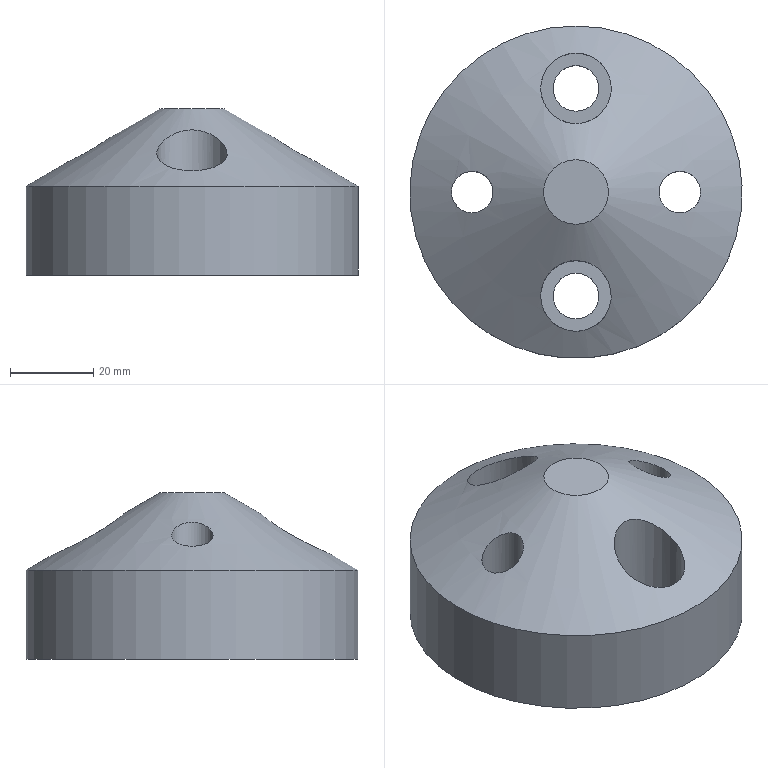Part | NX | features solid 2 | 1 solid | 12 faces | box 80 x 80 x 40 mm | volume 130381 mm3 | cylinder 7 | plane 4 | cone 1 | commonest cylinder face diameters 10 x2 11 x2 17 x2 80 x1
STEP:
#1=CARTESIAN_POINT('',(1255.,-150.,-35.));
#2=VERTEX_POINT('',#1);
#3=CARTESIAN_POINT('',(1255.,-155.,-35.));
#4=DIRECTION('',(0.,0.,1.));
#5=DIRECTION('',(0.,1.,0.));
#6=AXIS2_PLACEMENT_3D('',#3,#4,#5);
#7=CIRCLE('',#6,5.);
#8=EDGE_CURVE('',#2,#2,#7,.T.);
#9=ORIENTED_EDGE('',*,*,#8,.T.);
#10=EDGE_LOOP('',(#9));
#11=FACE_BOUND('',#10,.T.);
#12=CARTESIAN_POINT('',(1230.,-124.5,-35.));
#13=VERTEX_POINT('',#12);
#14=CARTESIAN_POINT('',(1230.,-130.,-35.));
#15=DIRECTION('',(0.,0.,1.));
#16=DIRECTION('',(0.,1.,0.));
#17=AXIS2_PLACEMENT_3D('',#14,#15,#16);
#18=CIRCLE('',#17,5.5);
#19=EDGE_CURVE('',#13,#13,#18,.T.);
#20=ORIENTED_EDGE('',*,*,#19,.T.);
#21=EDGE_LOOP('',(#20));
#22=FACE_BOUND('',#21,.T.);
#23=CARTESIAN_POINT('',(1230.,-115.,-35.));
#24=VERTEX_POINT('',#23);
#25=CARTESIAN_POINT('',(1230.,-155.,-35.));
#26=DIRECTION('',(0.,0.,1.));
#27=DIRECTION('',(0.,1.,0.));
#28=AXIS2_PLACEMENT_3D('',#25,#26,#27);
#29=CIRCLE('',#28,40.);
#30=EDGE_CURVE('',#24,#24,#29,.T.);
#31=ORIENTED_EDGE('',*,*,#30,.F.);
#32=EDGE_LOOP('',(#31));
#33=FACE_BOUND('',#32,.T.);
#34=CARTESIAN_POINT('',(1205.,-150.,-35.));
#35=VERTEX_POINT('',#34);
#36=CARTESIAN_POINT('',(1205.,-155.,-35.));
#37=DIRECTION('',(0.,0.,1.));
#38=DIRECTION('',(0.,1.,0.));
#39=AXIS2_PLACEMENT_3D('',#36,#37,#38);
#40=CIRCLE('',#39,5.);
#41=EDGE_CURVE('',#35,#35,#40,.T.);
#42=ORIENTED_EDGE('',*,*,#41,.T.);
#43=EDGE_LOOP('',(#42));
#44=FACE_BOUND('',#43,.T.);
#45=CARTESIAN_POINT('',(1230.,-174.5,-35.));
#46=VERTEX_POINT('',#45);
#47=CARTESIAN_POINT('',(1230.,-180.,-35.));
#48=DIRECTION('',(0.,0.,1.));
#49=DIRECTION('',(0.,1.,0.));
#50=AXIS2_PLACEMENT_3D('',#47,#48,#49);
#51=CIRCLE('',#50,5.5);
#52=EDGE_CURVE('',#46,#46,#51,.T.);
#53=ORIENTED_EDGE('',*,*,#52,.T.);
#54=EDGE_LOOP('',(#53));
#55=FACE_BOUND('',#54,.T.);
#56=CARTESIAN_POINT('',(1230.,-155.,-35.));
#57=DIRECTION('',(0.,0.,-1.));
#58=DIRECTION('',(0.,1.,0.));
#59=AXIS2_PLACEMENT_3D('',#56,#57,#58);
#60=PLANE('',#59);
#61=ADVANCED_FACE('',(#11,#22,#33,#44,#55),#60,.T.);
#62=CARTESIAN_POINT('',(1230.,-171.5,-25.));
#63=VERTEX_POINT('',#62);
#64=CARTESIAN_POINT('',(1230.,-180.,-25.));
#65=DIRECTION('',(0.,0.,1.));
#66=DIRECTION('',(0.,1.,0.));
#67=AXIS2_PLACEMENT_3D('',#64,#65,#66);
#68=CIRCLE('',#67,8.5);
#69=EDGE_CURVE('',#63,#63,#68,.T.);
#70=ORIENTED_EDGE('',*,*,#69,.T.);
#71=EDGE_LOOP('',(#70));
#72=FACE_BOUND('',#71,.T.);
#73=CARTESIAN_POINT('',(1230.,-174.5,-25.));
#74=VERTEX_POINT('',#73);
#75=CARTESIAN_POINT('',(1230.,-180.,-25.));
#76=DIRECTION('',(0.,0.,1.));
#77=DIRECTION('',(0.,1.,0.));
#78=AXIS2_PLACEMENT_3D('',#75,#76,#77);
#79=CIRCLE('',#78,5.5);
#80=EDGE_CURVE('',#74,#74,#79,.F.);
#81=ORIENTED_EDGE('',*,*,#80,.T.);
#82=EDGE_LOOP('',(#81));
#83=FACE_BOUND('',#82,.T.);
#84=CARTESIAN_POINT('',(1230.,-180.,-25.));
#85=DIRECTION('',(0.,0.,-1.));
#86=DIRECTION('',(0.,1.,0.));
#87=AXIS2_PLACEMENT_3D('',#84,#85,#86);
#88=PLANE('',#87);
#89=ADVANCED_FACE('',(#72,#83),#88,.F.);
#90=CARTESIAN_POINT('',(1230.,-147.206,5.));
#91=VERTEX_POINT('',#90);
#92=CARTESIAN_POINT('',(1230.,-155.,5.));
#93=DIRECTION('',(0.,0.,1.));
#94=DIRECTION('',(0.,1.,0.));
#95=AXIS2_PLACEMENT_3D('',#92,#93,#94);
#96=CIRCLE('',#95,7.794);
#97=EDGE_CURVE('',#91,#91,#96,.T.);
#98=ORIENTED_EDGE('',*,*,#97,.F.);
#99=EDGE_LOOP('',(#98));
#100=FACE_BOUND('',#99,.T.);
#101=CARTESIAN_POINT('',(1209.497,-157.186,-2.405));
#102=VERTEX_POINT('',#101);
#103=CARTESIAN_POINT('',(1210.155,-155.174,-1.934));
#104=CARTESIAN_POINT('',(1209.61,-157.276,-2.331));
#105=CARTESIAN_POINT('',(1208.388,-158.838,-3.169));
#106=CARTESIAN_POINT('',(1206.227,-160.117,-4.54));
#107=CARTESIAN_POINT('',(1202.995,-160.119,-6.355));
#108=CARTESIAN_POINT('',(1200.377,-157.688,-7.64));
#109=CARTESIAN_POINT('',(1199.848,-154.84,-7.893));
#110=CARTESIAN_POINT('',(1200.554,-152.03,-7.555));
#111=CARTESIAN_POINT('',(1203.307,-149.773,-6.193));
#112=CARTESIAN_POINT('',(1206.53,-149.966,-4.359));
#113=CARTESIAN_POINT('',(1208.617,-151.374,-3.016));
#114=CARTESIAN_POINT('',(1209.754,-153.037,-2.228));
#115=CARTESIAN_POINT('',(1210.155,-155.174,-1.934));
#116=CARTESIAN_POINT('',(1209.61,-157.276,-2.331));
#117=CARTESIAN_POINT('',(1208.388,-158.838,-3.169));
#118=B_SPLINE_CURVE_WITH_KNOTS('',3,(#103,#104,#105,#106,#107,#108,#109,#110,#111,#112,#113,#114,#115,#116,#117),.UNSPECIFIED.,.T.,.F.,(1,1,1,1,1,1,1,1,1,1,1,1,1,1,1,1,1,1,1),(-0.006313,-0.004209,-0.002104,0.,0.002104,0.004209,0.008418,0.01263,0.01473,0.01684,0.02104,0.02525,0.02736,0.02946,0.03157,0.03367,0.03577,0.03788,0.04209),.UNSPECIFIED.);
#119=EDGE_CURVE('',#102,#102,#118,.T.);
#120=ORIENTED_EDGE('',*,*,#119,.T.);
#121=EDGE_LOOP('',(#120));
#122=FACE_BOUND('',#121,.T.);
#123=CARTESIAN_POINT('',(1235.114,-136.79,-1.42));
#124=VERTEX_POINT('',#123);
#125=CARTESIAN_POINT('',(1237.421,-134.523,-3.074));
#126=CARTESIAN_POINT('',(1235.273,-136.934,-1.349));
#127=CARTESIAN_POINT('',(1232.172,-138.478,-0.05302));
#128=CARTESIAN_POINT('',(1228.448,-138.622,0.07805));
#129=CARTESIAN_POINT('',(1225.175,-137.259,-1.091));
#130=CARTESIAN_POINT('',(1222.878,-134.983,-2.765));
#131=CARTESIAN_POINT('',(1221.57,-132.108,-4.584));
#132=CARTESIAN_POINT('',(1221.289,-127.878,-6.935));
#133=CARTESIAN_POINT('',(1223.495,-123.689,-8.892));
#134=CARTESIAN_POINT('',(1227.812,-121.52,-9.833));
#135=CARTESIAN_POINT('',(1231.513,-121.371,-9.897));
#136=CARTESIAN_POINT('',(1234.898,-122.755,-9.299));
#137=CARTESIAN_POINT('',(1238.144,-126.114,-7.779));
#138=CARTESIAN_POINT('',(1238.927,-130.606,-5.499));
#139=CARTESIAN_POINT('',(1237.421,-134.523,-3.074));
#140=CARTESIAN_POINT('',(1235.273,-136.934,-1.349));
#141=CARTESIAN_POINT('',(1232.172,-138.478,-0.05302));
#142=B_SPLINE_CURVE_WITH_KNOTS('',3,(#125,#126,#127,#128,#129,#130,#131,#132,#133,#134,#135,#136,#137,#138,#139,#140,#141),.UNSPECIFIED.,.T.,.F.,(1,1,1,1,1,1,1,1,1,1,1,1,1,1,1,1,1,1,1,1,1),(-0.01435,-0.007177,-0.003588,0.,0.003588,0.007177,0.01077,0.01435,0.01794,0.02153,0.02871,0.0323,0.03588,0.03947,0.04306,0.05024,0.05383,0.05741,0.061,0.06459,0.06818),.UNSPECIFIED.);
#143=EDGE_CURVE('',#124,#124,#142,.T.);
#144=ORIENTED_EDGE('',*,*,#143,.T.);
#145=EDGE_LOOP('',(#144));
#146=FACE_BOUND('',#145,.T.);
#147=CARTESIAN_POINT('',(1230.,-115.,-13.594));
#148=VERTEX_POINT('',#147);
#149=CARTESIAN_POINT('',(1230.,-155.,-13.594));
#150=DIRECTION('',(0.,0.,1.));
#151=DIRECTION('',(0.,1.,0.));
#152=AXIS2_PLACEMENT_3D('',#149,#150,#151);
#153=CIRCLE('',#152,40.);
#154=EDGE_CURVE('',#148,#148,#153,.T.);
#155=ORIENTED_EDGE('',*,*,#154,.T.);
#156=EDGE_LOOP('',(#155));
#157=FACE_BOUND('',#156,.T.);
#158=CARTESIAN_POINT('',(1235.114,-173.21,-1.42));
#159=VERTEX_POINT('',#158);
#160=CARTESIAN_POINT('',(1232.159,-171.513,-0.04521));
#161=CARTESIAN_POINT('',(1235.279,-173.072,-1.354));
#162=CARTESIAN_POINT('',(1237.409,-175.461,-3.063));
#163=CARTESIAN_POINT('',(1238.927,-179.384,-5.493));
#164=CARTESIAN_POINT('',(1238.159,-183.841,-7.757));
#165=CARTESIAN_POINT('',(1234.948,-187.209,-9.283));
#166=CARTESIAN_POINT('',(1231.585,-188.614,-9.891));
#167=CARTESIAN_POINT('',(1227.892,-188.501,-9.842));
#168=CARTESIAN_POINT('',(1223.534,-186.361,-8.915));
#169=CARTESIAN_POINT('',(1221.293,-182.154,-6.951));
#170=CARTESIAN_POINT('',(1221.565,-177.912,-4.597));
#171=CARTESIAN_POINT('',(1222.864,-175.036,-2.778));
#172=CARTESIAN_POINT('',(1225.157,-172.755,-1.103));
#173=CARTESIAN_POINT('',(1228.405,-171.386,0.07106));
#174=CARTESIAN_POINT('',(1232.159,-171.513,-0.04521));
#175=CARTESIAN_POINT('',(1235.279,-173.072,-1.354));
#176=CARTESIAN_POINT('',(1237.409,-175.461,-3.063));
#177=B_SPLINE_CURVE_WITH_KNOTS('',3,(#160,#161,#162,#163,#164,#165,#166,#167,#168,#169,#170,#171,#172,#173,#174,#175,#176),.UNSPECIFIED.,.T.,.F.,(1,1,1,1,1,1,1,1,1,1,1,1,1,1,1,1,1,1,1,1,1),(-0.01073,-0.007151,-0.003576,0.,0.003576,0.007151,0.0143,0.01788,0.02145,0.02503,0.0286,0.03576,0.03933,0.04291,0.04648,0.05006,0.05363,0.05721,0.06079,0.06436,0.07151),.UNSPECIFIED.);
#178=EDGE_CURVE('',#159,#159,#177,.T.);
#179=ORIENTED_EDGE('',*,*,#178,.T.);
#180=EDGE_LOOP('',(#179));
#181=FACE_BOUND('',#180,.T.);
#182=CARTESIAN_POINT('',(1250.503,-157.186,-2.405));
#183=VERTEX_POINT('',#182);
#184=CARTESIAN_POINT('',(1251.618,-158.844,-3.173));
#185=CARTESIAN_POINT('',(1250.388,-157.271,-2.33));
#186=CARTESIAN_POINT('',(1249.848,-155.188,-1.936));
#187=CARTESIAN_POINT('',(1250.239,-153.051,-2.223));
#188=CARTESIAN_POINT('',(1251.376,-151.379,-3.012));
#189=CARTESIAN_POINT('',(1253.467,-149.966,-4.356));
#190=CARTESIAN_POINT('',(1256.682,-149.774,-6.187));
#191=CARTESIAN_POINT('',(1259.423,-152.003,-7.544));
#192=CARTESIAN_POINT('',(1260.151,-154.795,-7.893));
#193=CARTESIAN_POINT('',(1259.641,-157.665,-7.649));
#194=CARTESIAN_POINT('',(1257.017,-160.12,-6.362));
#195=CARTESIAN_POINT('',(1253.77,-160.114,-4.538));
#196=CARTESIAN_POINT('',(1251.618,-158.844,-3.173));
#197=CARTESIAN_POINT('',(1250.388,-157.271,-2.33));
#198=CARTESIAN_POINT('',(1249.848,-155.188,-1.936));
#199=B_SPLINE_CURVE_WITH_KNOTS('',3,(#184,#185,#186,#187,#188,#189,#190,#191,#192,#193,#194,#195,#196,#197,#198),.UNSPECIFIED.,.T.,.F.,(1,1,1,1,1,1,1,1,1,1,1,1,1,1,1,1,1,1,1),(-0.008443,-0.004222,-0.002111,0.,0.002111,0.004222,0.006333,0.008443,0.01267,0.01689,0.019,0.02111,0.02533,0.02955,0.03166,0.03377,0.03588,0.038,0.04011),.UNSPECIFIED.);
#200=EDGE_CURVE('',#183,#183,#199,.T.);
#201=ORIENTED_EDGE('',*,*,#200,.T.);
#202=EDGE_LOOP('',(#201));
#203=FACE_BOUND('',#202,.T.);
#204=CARTESIAN_POINT('',(1230.,-155.,-13.594));
#205=DIRECTION('',(0.,0.,-1.));
#206=DIRECTION('',(0.,1.,0.));
#207=AXIS2_PLACEMENT_3D('',#204,#205,#206);
#208=CONICAL_SURFACE('',#207,40.,1.047);
#209=ADVANCED_FACE('',(#100,#122,#146,#157,#181,#203),#208,.T.);
#210=CARTESIAN_POINT('',(1230.,-121.5,-25.));
#211=VERTEX_POINT('',#210);
#212=CARTESIAN_POINT('',(1230.,-130.,-25.));
#213=DIRECTION('',(0.,0.,1.));
#214=DIRECTION('',(0.,1.,0.));
#215=AXIS2_PLACEMENT_3D('',#212,#213,#214);
#216=CIRCLE('',#215,8.5);
#217=EDGE_CURVE('',#211,#211,#216,.T.);
#218=ORIENTED_EDGE('',*,*,#217,.T.);
#219=EDGE_LOOP('',(#218));
#220=FACE_BOUND('',#219,.T.);
#221=CARTESIAN_POINT('',(1230.,-124.5,-25.));
#222=VERTEX_POINT('',#221);
#223=CARTESIAN_POINT('',(1230.,-130.,-25.));
#224=DIRECTION('',(0.,0.,1.));
#225=DIRECTION('',(0.,1.,0.));
#226=AXIS2_PLACEMENT_3D('',#223,#224,#225);
#227=CIRCLE('',#226,5.5);
#228=EDGE_CURVE('',#222,#222,#227,.F.);
#229=ORIENTED_EDGE('',*,*,#228,.T.);
#230=EDGE_LOOP('',(#229));
#231=FACE_BOUND('',#230,.T.);
#232=CARTESIAN_POINT('',(1230.,-130.,-25.));
#233=DIRECTION('',(0.,0.,-1.));
#234=DIRECTION('',(0.,1.,0.));
#235=AXIS2_PLACEMENT_3D('',#232,#233,#234);
#236=PLANE('',#235);
#237=ADVANCED_FACE('',(#220,#231),#236,.F.);
#238=ORIENTED_EDGE('',*,*,#154,.F.);
#239=EDGE_LOOP('',(#238));
#240=FACE_BOUND('',#239,.T.);
#241=ORIENTED_EDGE('',*,*,#30,.T.);
#242=EDGE_LOOP('',(#241));
#243=FACE_BOUND('',#242,.T.);
#244=CARTESIAN_POINT('',(1230.,-155.,131.744));
#245=DIRECTION('',(0.,0.,-1.));
#246=DIRECTION('',(0.,1.,0.));
#247=AXIS2_PLACEMENT_3D('',#244,#245,#246);
#248=CYLINDRICAL_SURFACE('',#247,40.);
#249=ADVANCED_FACE('',(#240,#243),#248,.T.);
#250=ORIENTED_EDGE('',*,*,#217,.F.);
#251=EDGE_LOOP('',(#250));
#252=FACE_BOUND('',#251,.T.);
#253=ORIENTED_EDGE('',*,*,#143,.F.);
#254=EDGE_LOOP('',(#253));
#255=FACE_BOUND('',#254,.T.);
#256=CARTESIAN_POINT('',(1230.,-130.,-25.));
#257=DIRECTION('',(0.,0.,1.));
#258=DIRECTION('',(0.,-1.,0.));
#259=AXIS2_PLACEMENT_3D('',#256,#257,#258);
#260=CYLINDRICAL_SURFACE('',#259,8.5);
#261=ADVANCED_FACE('',(#252,#255),#260,.F.);
#262=ORIENTED_EDGE('',*,*,#69,.F.);
#263=EDGE_LOOP('',(#262));
#264=FACE_BOUND('',#263,.T.);
#265=ORIENTED_EDGE('',*,*,#178,.F.);
#266=EDGE_LOOP('',(#265));
#267=FACE_BOUND('',#266,.T.);
#268=CARTESIAN_POINT('',(1230.,-180.,-25.));
#269=DIRECTION('',(0.,0.,1.));
#270=DIRECTION('',(0.,-1.,0.));
#271=AXIS2_PLACEMENT_3D('',#268,#269,#270);
#272=CYLINDRICAL_SURFACE('',#271,8.5);
#273=ADVANCED_FACE('',(#264,#267),#272,.F.);
#274=ORIENTED_EDGE('',*,*,#19,.F.);
#275=EDGE_LOOP('',(#274));
#276=FACE_BOUND('',#275,.T.);
#277=ORIENTED_EDGE('',*,*,#228,.F.);
#278=EDGE_LOOP('',(#277));
#279=FACE_BOUND('',#278,.T.);
#280=CARTESIAN_POINT('',(1230.,-130.,-35.));
#281=DIRECTION('',(0.,0.,1.));
#282=DIRECTION('',(0.,-1.,0.));
#283=AXIS2_PLACEMENT_3D('',#280,#281,#282);
#284=CYLINDRICAL_SURFACE('',#283,5.5);
#285=ADVANCED_FACE('',(#276,#279),#284,.F.);
#286=ORIENTED_EDGE('',*,*,#41,.F.);
#287=EDGE_LOOP('',(#286));
#288=FACE_BOUND('',#287,.T.);
#289=ORIENTED_EDGE('',*,*,#119,.F.);
#290=EDGE_LOOP('',(#289));
#291=FACE_BOUND('',#290,.T.);
#292=CARTESIAN_POINT('',(1205.,-155.,-35.));
#293=DIRECTION('',(0.,0.,1.));
#294=DIRECTION('',(0.,-1.,0.));
#295=AXIS2_PLACEMENT_3D('',#292,#293,#294);
#296=CYLINDRICAL_SURFACE('',#295,5.);
#297=ADVANCED_FACE('',(#288,#291),#296,.F.);
#298=ORIENTED_EDGE('',*,*,#8,.F.);
#299=EDGE_LOOP('',(#298));
#300=FACE_BOUND('',#299,.T.);
#301=ORIENTED_EDGE('',*,*,#200,.F.);
#302=EDGE_LOOP('',(#301));
#303=FACE_BOUND('',#302,.T.);
#304=CARTESIAN_POINT('',(1255.,-155.,-35.));
#305=DIRECTION('',(0.,0.,1.));
#306=DIRECTION('',(0.,-1.,0.));
#307=AXIS2_PLACEMENT_3D('',#304,#305,#306);
#308=CYLINDRICAL_SURFACE('',#307,5.);
#309=ADVANCED_FACE('',(#300,#303),#308,.F.);
#310=ORIENTED_EDGE('',*,*,#52,.F.);
#311=EDGE_LOOP('',(#310));
#312=FACE_BOUND('',#311,.T.);
#313=ORIENTED_EDGE('',*,*,#80,.F.);
#314=EDGE_LOOP('',(#313));
#315=FACE_BOUND('',#314,.T.);
#316=CARTESIAN_POINT('',(1230.,-180.,-35.));
#317=DIRECTION('',(0.,0.,1.));
#318=DIRECTION('',(0.,-1.,0.));
#319=AXIS2_PLACEMENT_3D('',#316,#317,#318);
#320=CYLINDRICAL_SURFACE('',#319,5.5);
#321=ADVANCED_FACE('',(#312,#315),#320,.F.);
#322=ORIENTED_EDGE('',*,*,#97,.T.);
#323=EDGE_LOOP('',(#322));
#324=FACE_BOUND('',#323,.T.);
#325=CARTESIAN_POINT('',(1230.,-155.,5.));
#326=DIRECTION('',(0.,0.,-1.));
#327=DIRECTION('',(0.,1.,0.));
#328=AXIS2_PLACEMENT_3D('',#325,#326,#327);
#329=PLANE('',#328);
#330=ADVANCED_FACE('',(#324),#329,.F.);
#331=CLOSED_SHELL('',(#61,#89,#209,#237,#249,#261,#273,#285,#297,#309,#321,#330));
#332=MANIFOLD_SOLID_BREP('',#331);
#333=(LENGTH_UNIT()NAMED_UNIT(*)SI_UNIT(.MILLI.,.METRE.));
#334=UNCERTAINTY_MEASURE_WITH_UNIT(LENGTH_MEASURE(0.0508),#333,'','');
#335=(NAMED_UNIT(*)PLANE_ANGLE_UNIT()SI_UNIT($,.RADIAN.));
#336=(NAMED_UNIT(*)SI_UNIT($,.STERADIAN.)SOLID_ANGLE_UNIT());
#337=(GEOMETRIC_REPRESENTATION_CONTEXT(3)GLOBAL_UNCERTAINTY_ASSIGNED_CONTEXT((#334))GLOBAL_UNIT_ASSIGNED_CONTEXT((#333,#335,#336))REPRESENTATION_CONTEXT('',''));
#338=ADVANCED_BREP_SHAPE_REPRESENTATION('',(#332),#337);